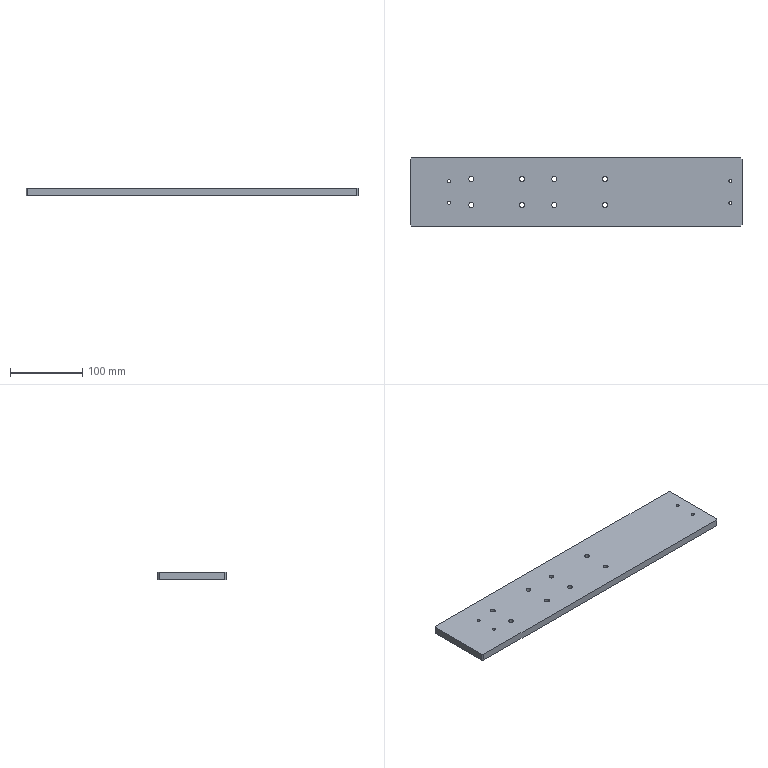Part | STEP file | 001-004-Feeding mechanism feed base plate | 1 solid | 34 faces | box 460 x 95 x 10 mm | volume 433460 mm3 | cylinder 24 | plane 10 | commonest cylinder face diameters 6.8 x16 4.2 x8